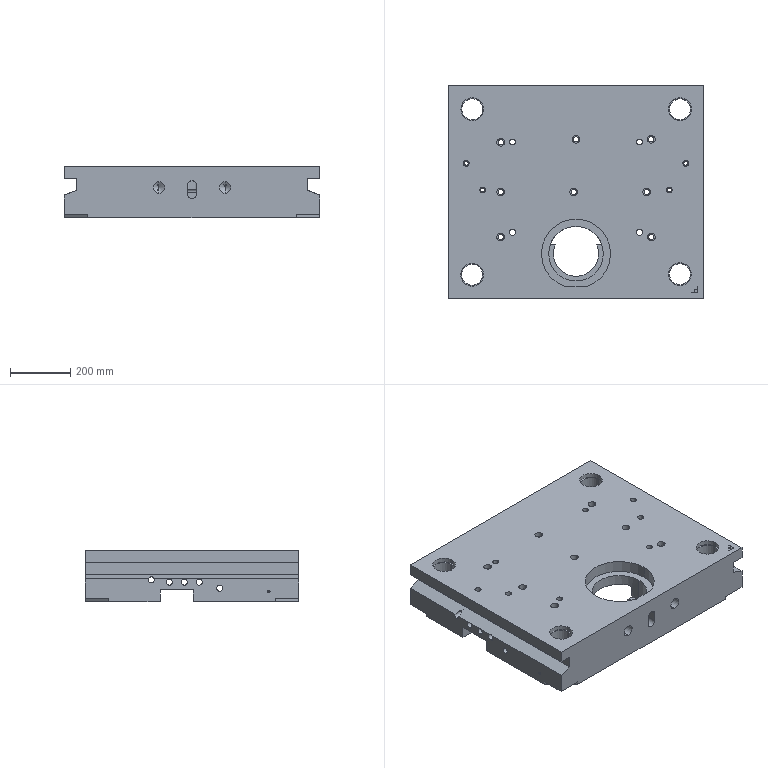Part | SolidWorks | features BaseBody 1 | 1 solid | 338 faces | box 850 x 710 x 170 mm | volume 68222624 mm3 | cylinder 191 | plane 99 | cone 28 | torus 8 | spline 8 | sphere 4 | commonest cylinder face diameters 20 x43 10 x23 6.8 x16 18 x16 26 x16 9 x8